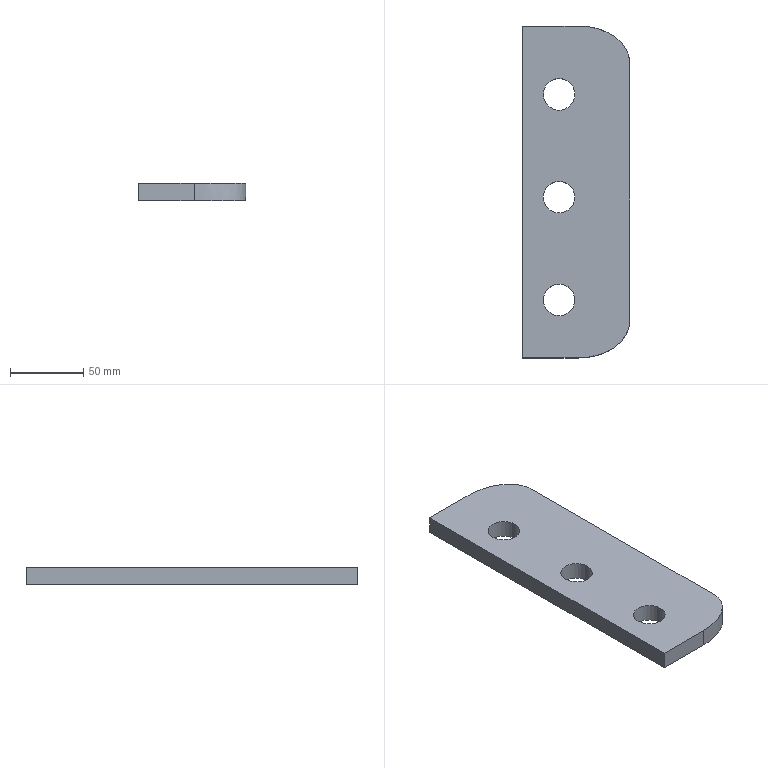Part | STEP file | PN_0022 channel connecting plate 12t_Default<As Machined> | 1 solid | 11 faces | box 73 x 226 x 12 mm | volume 180413 mm3 | plane 6 | cylinder 3 | spline 2 | commonest cylinder face diameters 21.5 x3